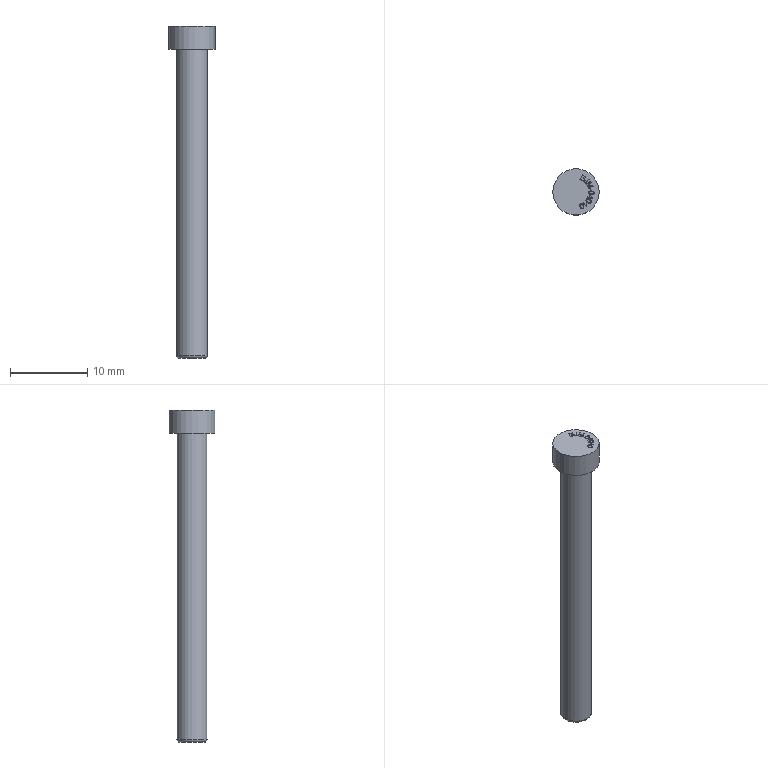Part | STEP file | lll_id654_x_t | 1 solid | 95 faces | box 6 x 6 x 43 mm | volume 587 mm3 | plane 74 | other 18 | cylinder 2 | torus 1 | commonest cylinder face diameters 4 x1 6 x1